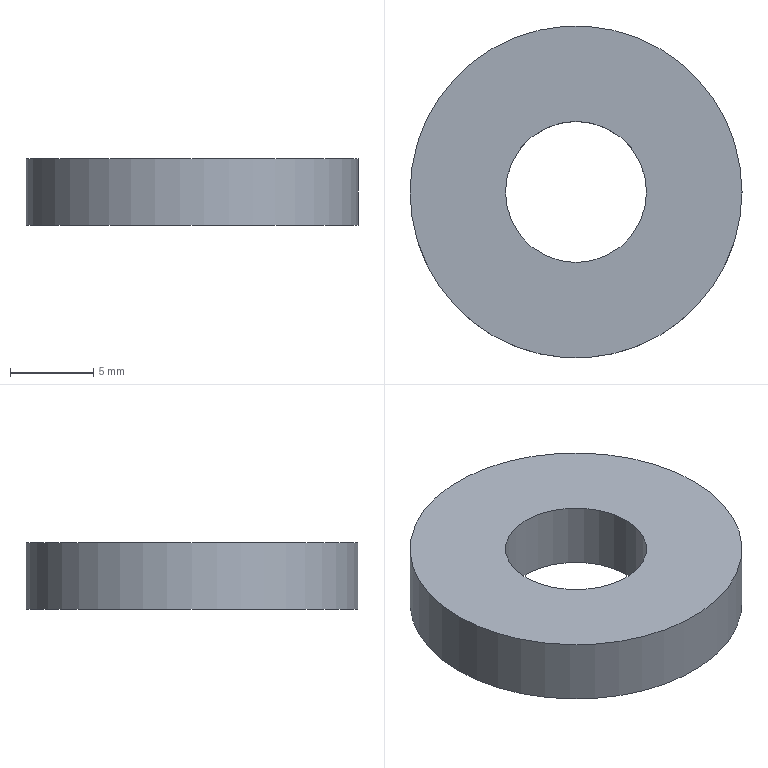Part | STEP file | YBQDJ-PD-24 | 1 solid | 4 faces | box 20 x 20 x 4 mm | volume 1030 mm3 | plane 2 | cylinder 2 | commonest cylinder face diameters 8.5 x1 20 x1
STEP:
#1=CARTESIAN_POINT('',(0.,0.,0.));
#2=DIRECTION('',(0.,0.,1.));
#3=DIRECTION('',(1.,0.,0.));
#4=AXIS2_PLACEMENT_3D('',#1,#2,#3);
#5=CARTESIAN_POINT('',(-281.5,391.,149.2));
#6=VERTEX_POINT('',#5);
#7=CARTESIAN_POINT('',(-271.5,391.,149.2));
#8=DIRECTION('',(0.,0.,1.));
#9=DIRECTION('',(-1.,0.,0.));
#10=AXIS2_PLACEMENT_3D('',#7,#8,#9);
#11=CIRCLE('',#10,10.);
#12=CARTESIAN_POINT('',(-271.5,391.,149.2));
#13=DIRECTION('',(0.,0.,-1.));
#14=DIRECTION('',(-1.,0.,0.));
#15=AXIS2_PLACEMENT_3D('',#12,#13,#14);
#16=PLANE('',#15);
#17=CARTESIAN_POINT('',(10.,0.));
#18=CARTESIAN_POINT('',(10.,-17.321));
#19=CARTESIAN_POINT('',(-5.,-8.66));
#20=CARTESIAN_POINT('',(-20.,0.));
#21=CARTESIAN_POINT('',(-5.,8.66));
#22=CARTESIAN_POINT('',(10.,17.321));
#23=CARTESIAN_POINT('',(10.,0.));
#24=(BOUNDED_CURVE()B_SPLINE_CURVE(2,(#17,#18,#19,#20,#21,#22,#23),.UNSPECIFIED.,.T.,.F.)B_SPLINE_CURVE_WITH_KNOTS((1,2,2,2,2,1),(-2.094,0.,2.094,4.189,6.283,8.378),.UNSPECIFIED.)CURVE()GEOMETRIC_REPRESENTATION_ITEM()RATIONAL_B_SPLINE_CURVE((1.,0.5,1.,0.5,1.,0.5,1.))REPRESENTATION_ITEM(''));
#25=(GEOMETRIC_REPRESENTATION_CONTEXT(2)PARAMETRIC_REPRESENTATION_CONTEXT()REPRESENTATION_CONTEXT('',''));
#26=DEFINITIONAL_REPRESENTATION('',(#24),#25);
#27=PCURVE('',#16,#26);
#28=CARTESIAN_POINT('',(-271.5,391.,149.2));
#29=DIRECTION('',(0.,0.,1.));
#30=DIRECTION('',(1.,0.,0.));
#31=AXIS2_PLACEMENT_3D('',#28,#29,#30);
#32=CYLINDRICAL_SURFACE('',#31,10.);
#33=CARTESIAN_POINT('',(3.142,0.));
#34=DIRECTION('',(1.,0.));
#35=VECTOR('',#34,1.);
#36=LINE('',#33,#35);
#37=(GEOMETRIC_REPRESENTATION_CONTEXT(2)PARAMETRIC_REPRESENTATION_CONTEXT()REPRESENTATION_CONTEXT('',''));
#38=DEFINITIONAL_REPRESENTATION('',(#36),#37);
#39=PCURVE('',#32,#38);
#40=SURFACE_CURVE('',#11,(#27,#39),.PCURVE_S1.);
#41=EDGE_CURVE('',#6,#6,#40,.T.);
#42=ORIENTED_EDGE('',*,*,#41,.F.);
#43=EDGE_LOOP('',(#42));
#44=FACE_BOUND('',#43,.T.);
#45=CARTESIAN_POINT('',(-275.75,391.,149.2));
#46=VERTEX_POINT('',#45);
#47=CARTESIAN_POINT('',(-271.5,391.,149.2));
#48=DIRECTION('',(0.,0.,1.));
#49=DIRECTION('',(-1.,0.,0.));
#50=AXIS2_PLACEMENT_3D('',#47,#48,#49);
#51=CIRCLE('',#50,4.25);
#52=CARTESIAN_POINT('',(4.25,0.));
#53=CARTESIAN_POINT('',(4.25,-7.361));
#54=CARTESIAN_POINT('',(-2.125,-3.681));
#55=CARTESIAN_POINT('',(-8.5,0.));
#56=CARTESIAN_POINT('',(-2.125,3.681));
#57=CARTESIAN_POINT('',(4.25,7.361));
#58=CARTESIAN_POINT('',(4.25,0.));
#59=(BOUNDED_CURVE()B_SPLINE_CURVE(2,(#52,#53,#54,#55,#56,#57,#58),.UNSPECIFIED.,.T.,.F.)B_SPLINE_CURVE_WITH_KNOTS((1,2,2,2,2,1),(-2.094,0.,2.094,4.189,6.283,8.378),.UNSPECIFIED.)CURVE()GEOMETRIC_REPRESENTATION_ITEM()RATIONAL_B_SPLINE_CURVE((1.,0.5,1.,0.5,1.,0.5,1.))REPRESENTATION_ITEM(''));
#60=(GEOMETRIC_REPRESENTATION_CONTEXT(2)PARAMETRIC_REPRESENTATION_CONTEXT()REPRESENTATION_CONTEXT('',''));
#61=DEFINITIONAL_REPRESENTATION('',(#59),#60);
#62=PCURVE('',#16,#61);
#63=CARTESIAN_POINT('',(-271.5,391.,149.2));
#64=DIRECTION('',(0.,0.,1.));
#65=DIRECTION('',(1.,0.,0.));
#66=AXIS2_PLACEMENT_3D('',#63,#64,#65);
#67=CYLINDRICAL_SURFACE('',#66,4.25);
#68=CARTESIAN_POINT('',(3.142,0.));
#69=DIRECTION('',(1.,0.));
#70=VECTOR('',#69,1.);
#71=LINE('',#68,#70);
#72=(GEOMETRIC_REPRESENTATION_CONTEXT(2)PARAMETRIC_REPRESENTATION_CONTEXT()REPRESENTATION_CONTEXT('',''));
#73=DEFINITIONAL_REPRESENTATION('',(#71),#72);
#74=PCURVE('',#67,#73);
#75=SURFACE_CURVE('',#51,(#62,#74),.PCURVE_S1.);
#76=EDGE_CURVE('',#46,#46,#75,.T.);
#77=ORIENTED_EDGE('',*,*,#76,.T.);
#78=EDGE_LOOP('',(#77));
#79=FACE_BOUND('',#78,.T.);
#80=ADVANCED_FACE('',(#44,#79),#16,.T.);
#81=CARTESIAN_POINT('',(-281.5,391.,153.2));
#82=VERTEX_POINT('',#81);
#83=CARTESIAN_POINT('',(-271.5,391.,153.2));
#84=DIRECTION('',(0.,0.,1.));
#85=DIRECTION('',(-1.,0.,0.));
#86=AXIS2_PLACEMENT_3D('',#83,#84,#85);
#87=CIRCLE('',#86,10.);
#88=CARTESIAN_POINT('',(-271.5,391.,153.2));
#89=DIRECTION('',(0.,0.,-1.));
#90=DIRECTION('',(-1.,0.,0.));
#91=AXIS2_PLACEMENT_3D('',#88,#89,#90);
#92=PLANE('',#91);
#93=CARTESIAN_POINT('',(10.,0.));
#94=CARTESIAN_POINT('',(10.,-17.321));
#95=CARTESIAN_POINT('',(-5.,-8.66));
#96=CARTESIAN_POINT('',(-20.,0.));
#97=CARTESIAN_POINT('',(-5.,8.66));
#98=CARTESIAN_POINT('',(10.,17.321));
#99=CARTESIAN_POINT('',(10.,0.));
#100=(BOUNDED_CURVE()B_SPLINE_CURVE(2,(#93,#94,#95,#96,#97,#98,#99),.UNSPECIFIED.,.T.,.F.)B_SPLINE_CURVE_WITH_KNOTS((1,2,2,2,2,1),(-2.094,0.,2.094,4.189,6.283,8.378),.UNSPECIFIED.)CURVE()GEOMETRIC_REPRESENTATION_ITEM()RATIONAL_B_SPLINE_CURVE((1.,0.5,1.,0.5,1.,0.5,1.))REPRESENTATION_ITEM(''));
#101=(GEOMETRIC_REPRESENTATION_CONTEXT(2)PARAMETRIC_REPRESENTATION_CONTEXT()REPRESENTATION_CONTEXT('',''));
#102=DEFINITIONAL_REPRESENTATION('',(#100),#101);
#103=PCURVE('',#92,#102);
#104=CARTESIAN_POINT('',(3.142,4.));
#105=DIRECTION('',(1.,0.));
#106=VECTOR('',#105,1.);
#107=LINE('',#104,#106);
#108=(GEOMETRIC_REPRESENTATION_CONTEXT(2)PARAMETRIC_REPRESENTATION_CONTEXT()REPRESENTATION_CONTEXT('',''));
#109=DEFINITIONAL_REPRESENTATION('',(#107),#108);
#110=PCURVE('',#32,#109);
#111=SURFACE_CURVE('',#87,(#103,#110),.PCURVE_S1.);
#112=EDGE_CURVE('',#82,#82,#111,.T.);
#113=ORIENTED_EDGE('',*,*,#112,.T.);
#114=EDGE_LOOP('',(#113));
#115=FACE_BOUND('',#114,.T.);
#116=CARTESIAN_POINT('',(-275.75,391.,153.2));
#117=VERTEX_POINT('',#116);
#118=CARTESIAN_POINT('',(-271.5,391.,153.2));
#119=DIRECTION('',(0.,0.,1.));
#120=DIRECTION('',(-1.,0.,0.));
#121=AXIS2_PLACEMENT_3D('',#118,#119,#120);
#122=CIRCLE('',#121,4.25);
#123=CARTESIAN_POINT('',(4.25,0.));
#124=CARTESIAN_POINT('',(4.25,-7.361));
#125=CARTESIAN_POINT('',(-2.125,-3.681));
#126=CARTESIAN_POINT('',(-8.5,0.));
#127=CARTESIAN_POINT('',(-2.125,3.681));
#128=CARTESIAN_POINT('',(4.25,7.361));
#129=CARTESIAN_POINT('',(4.25,0.));
#130=(BOUNDED_CURVE()B_SPLINE_CURVE(2,(#123,#124,#125,#126,#127,#128,#129),.UNSPECIFIED.,.T.,.F.)B_SPLINE_CURVE_WITH_KNOTS((1,2,2,2,2,1),(-2.094,0.,2.094,4.189,6.283,8.378),.UNSPECIFIED.)CURVE()GEOMETRIC_REPRESENTATION_ITEM()RATIONAL_B_SPLINE_CURVE((1.,0.5,1.,0.5,1.,0.5,1.))REPRESENTATION_ITEM(''));
#131=(GEOMETRIC_REPRESENTATION_CONTEXT(2)PARAMETRIC_REPRESENTATION_CONTEXT()REPRESENTATION_CONTEXT('',''));
#132=DEFINITIONAL_REPRESENTATION('',(#130),#131);
#133=PCURVE('',#92,#132);
#134=CARTESIAN_POINT('',(3.142,4.));
#135=DIRECTION('',(1.,0.));
#136=VECTOR('',#135,1.);
#137=LINE('',#134,#136);
#138=(GEOMETRIC_REPRESENTATION_CONTEXT(2)PARAMETRIC_REPRESENTATION_CONTEXT()REPRESENTATION_CONTEXT('',''));
#139=DEFINITIONAL_REPRESENTATION('',(#137),#138);
#140=PCURVE('',#67,#139);
#141=SURFACE_CURVE('',#122,(#133,#140),.PCURVE_S1.);
#142=EDGE_CURVE('',#117,#117,#141,.T.);
#143=ORIENTED_EDGE('',*,*,#142,.F.);
#144=EDGE_LOOP('',(#143));
#145=FACE_BOUND('',#144,.T.);
#146=ADVANCED_FACE('',(#115,#145),#92,.F.);
#147=ORIENTED_EDGE('',*,*,#41,.T.);
#148=CARTESIAN_POINT('',(-281.5,391.,149.2));
#149=CARTESIAN_POINT('',(-281.5,391.,153.2));
#150=B_SPLINE_CURVE_WITH_KNOTS('',1,(#148,#149),.UNSPECIFIED.,.F.,.F.,(2,2),(0.,4.),.PIECEWISE_BEZIER_KNOTS.);
#151=CARTESIAN_POINT('',(9.425,0.));
#152=DIRECTION('',(0.,1.));
#153=VECTOR('',#152,1.);
#154=LINE('',#151,#153);
#155=(GEOMETRIC_REPRESENTATION_CONTEXT(2)PARAMETRIC_REPRESENTATION_CONTEXT()REPRESENTATION_CONTEXT('',''));
#156=DEFINITIONAL_REPRESENTATION('',(#154),#155);
#157=PCURVE('',#32,#156);
#158=CARTESIAN_POINT('',(3.142,0.));
#159=DIRECTION('',(0.,1.));
#160=VECTOR('',#159,1.);
#161=LINE('',#158,#160);
#162=(GEOMETRIC_REPRESENTATION_CONTEXT(2)PARAMETRIC_REPRESENTATION_CONTEXT()REPRESENTATION_CONTEXT('',''));
#163=DEFINITIONAL_REPRESENTATION('',(#161),#162);
#164=PCURVE('',#32,#163);
#165=SEAM_CURVE('',#150,(#157,#164),.PCURVE_S1.);
#166=EDGE_CURVE('',#6,#82,#165,.T.);
#167=ORIENTED_EDGE('',*,*,#166,.T.);
#168=ORIENTED_EDGE('',*,*,#112,.F.);
#169=ORIENTED_EDGE('',*,*,#166,.F.);
#170=EDGE_LOOP('',(#147,#167,#168,#169));
#171=FACE_BOUND('',#170,.T.);
#172=ADVANCED_FACE('',(#171),#32,.T.);
#173=ORIENTED_EDGE('',*,*,#76,.T.);
#174=CARTESIAN_POINT('',(-275.75,391.,149.2));
#175=CARTESIAN_POINT('',(-275.75,391.,153.2));
#176=B_SPLINE_CURVE_WITH_KNOTS('',1,(#174,#175),.UNSPECIFIED.,.F.,.F.,(2,2),(0.,4.),.PIECEWISE_BEZIER_KNOTS.);
#177=CARTESIAN_POINT('',(9.425,0.));
#178=DIRECTION('',(0.,1.));
#179=VECTOR('',#178,1.);
#180=LINE('',#177,#179);
#181=(GEOMETRIC_REPRESENTATION_CONTEXT(2)PARAMETRIC_REPRESENTATION_CONTEXT()REPRESENTATION_CONTEXT('',''));
#182=DEFINITIONAL_REPRESENTATION('',(#180),#181);
#183=PCURVE('',#67,#182);
#184=CARTESIAN_POINT('',(3.142,0.));
#185=DIRECTION('',(0.,1.));
#186=VECTOR('',#185,1.);
#187=LINE('',#184,#186);
#188=(GEOMETRIC_REPRESENTATION_CONTEXT(2)PARAMETRIC_REPRESENTATION_CONTEXT()REPRESENTATION_CONTEXT('',''));
#189=DEFINITIONAL_REPRESENTATION('',(#187),#188);
#190=PCURVE('',#67,#189);
#191=SEAM_CURVE('',#176,(#183,#190),.PCURVE_S1.);
#192=EDGE_CURVE('',#46,#117,#191,.T.);
#193=ORIENTED_EDGE('',*,*,#192,.T.);
#194=ORIENTED_EDGE('',*,*,#142,.F.);
#195=ORIENTED_EDGE('',*,*,#192,.F.);
#196=EDGE_LOOP('',(#173,#193,#194,#195));
#197=FACE_BOUND('',#196,.F.);
#198=ADVANCED_FACE('',(#197),#67,.F.);
#199=CLOSED_SHELL('',(#80,#146,#172,#198));
#200=MANIFOLD_SOLID_BREP('',#199);
#201=(LENGTH_UNIT()NAMED_UNIT(*)SI_UNIT(.MILLI.,.METRE.));
#202=UNCERTAINTY_MEASURE_WITH_UNIT(LENGTH_MEASURE(0.00001),#201,'','');
#203=(NAMED_UNIT(*)PLANE_ANGLE_UNIT()SI_UNIT($,.RADIAN.));
#204=(NAMED_UNIT(*)SI_UNIT($,.STERADIAN.)SOLID_ANGLE_UNIT());
#205=(GEOMETRIC_REPRESENTATION_CONTEXT(3)GLOBAL_UNCERTAINTY_ASSIGNED_CONTEXT((#202))GLOBAL_UNIT_ASSIGNED_CONTEXT((#201,#203,#204))REPRESENTATION_CONTEXT('',''));
#206=ADVANCED_BREP_SHAPE_REPRESENTATION('',(#4,#200),#205);